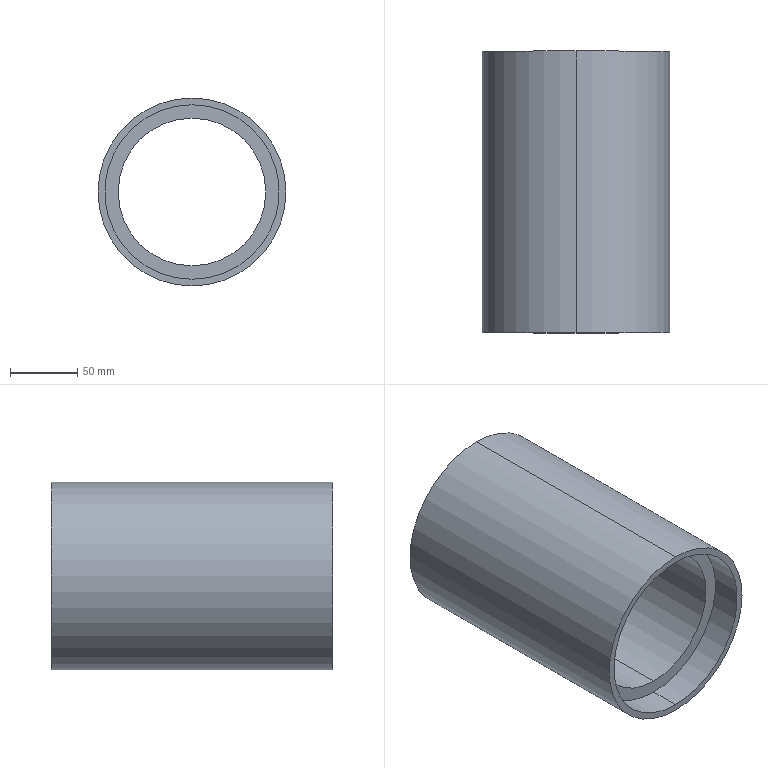Part | SolidWorks | features BaseBody 1 | 1 solid | 12 faces | box 140 x 210 x 140 mm | volume 1063586 mm3 | cylinder 8 | plane 4 | commonest cylinder face diameters 130 x4 110 x2 140 x2
STEP:
#1=CARTESIAN_POINT('',(0.,187.,-55.));
#2=VERTEX_POINT('',#1);
#3=CARTESIAN_POINT('',(0.,187.,55.));
#4=VERTEX_POINT('',#3);
#5=CARTESIAN_POINT('',(0.,187.,0.));
#6=DIRECTION('',(0.,1.,0.));
#7=DIRECTION('',(0.,0.,1.));
#8=AXIS2_PLACEMENT_3D('',#5,#6,#7);
#9=CIRCLE('',#8,55.);
#10=EDGE_CURVE('',#2,#4,#9,.T.);
#11=ORIENTED_EDGE('',*,*,#10,.T.);
#12=CARTESIAN_POINT('',(0.,23.,55.));
#13=VERTEX_POINT('',#12);
#14=CARTESIAN_POINT('',(0.,210.,55.));
#15=DIRECTION('',(0.,-1.,0.));
#16=VECTOR('',#15,1000.);
#17=LINE('',#14,#16);
#18=EDGE_CURVE('',#4,#13,#17,.T.);
#19=ORIENTED_EDGE('',*,*,#18,.T.);
#20=CARTESIAN_POINT('',(0.,23.,-55.));
#21=VERTEX_POINT('',#20);
#22=CARTESIAN_POINT('',(0.,23.,0.));
#23=DIRECTION('',(0.,-1.,0.));
#24=DIRECTION('',(0.,0.,-1.));
#25=AXIS2_PLACEMENT_3D('',#22,#23,#24);
#26=CIRCLE('',#25,55.);
#27=EDGE_CURVE('',#13,#21,#26,.T.);
#28=ORIENTED_EDGE('',*,*,#27,.T.);
#29=CARTESIAN_POINT('',(0.,210.,-55.));
#30=DIRECTION('',(0.,-1.,0.));
#31=VECTOR('',#30,1000.);
#32=LINE('',#29,#31);
#33=EDGE_CURVE('',#2,#21,#32,.T.);
#34=ORIENTED_EDGE('',*,*,#33,.F.);
#35=EDGE_LOOP('',(#11,#19,#28,#34));
#36=FACE_OUTER_BOUND('',#35,.T.);
#37=CARTESIAN_POINT('',(0.,210.,0.));
#38=DIRECTION('',(0.,-1.,0.));
#39=DIRECTION('',(0.,0.,-1.));
#40=AXIS2_PLACEMENT_3D('',#37,#38,#39);
#41=CYLINDRICAL_SURFACE('',#40,55.);
#42=ADVANCED_FACE('',(#36),#41,.F.);
#43=CARTESIAN_POINT('',(0.,23.,65.));
#44=VERTEX_POINT('',#43);
#45=CARTESIAN_POINT('',(0.,23.,-65.));
#46=VERTEX_POINT('',#45);
#47=CARTESIAN_POINT('',(0.,23.,0.));
#48=DIRECTION('',(0.,-1.,0.));
#49=DIRECTION('',(0.,0.,-1.));
#50=AXIS2_PLACEMENT_3D('',#47,#48,#49);
#51=CIRCLE('',#50,65.);
#52=EDGE_CURVE('',#44,#46,#51,.T.);
#53=ORIENTED_EDGE('',*,*,#52,.F.);
#54=CARTESIAN_POINT('',(0.,0.,65.));
#55=VERTEX_POINT('',#54);
#56=CARTESIAN_POINT('',(0.,23.,65.));
#57=DIRECTION('',(0.,-1.,0.));
#58=VECTOR('',#57,1000.);
#59=LINE('',#56,#58);
#60=EDGE_CURVE('',#44,#55,#59,.T.);
#61=ORIENTED_EDGE('',*,*,#60,.T.);
#62=CARTESIAN_POINT('',(0.,0.,-65.));
#63=VERTEX_POINT('',#62);
#64=CARTESIAN_POINT('',(0.,0.,0.));
#65=DIRECTION('',(0.,-1.,0.));
#66=DIRECTION('',(0.,0.,-1.));
#67=AXIS2_PLACEMENT_3D('',#64,#65,#66);
#68=CIRCLE('',#67,65.);
#69=EDGE_CURVE('',#55,#63,#68,.T.);
#70=ORIENTED_EDGE('',*,*,#69,.T.);
#71=CARTESIAN_POINT('',(0.,23.,-65.));
#72=DIRECTION('',(0.,-1.,0.));
#73=VECTOR('',#72,1000.);
#74=LINE('',#71,#73);
#75=EDGE_CURVE('',#46,#63,#74,.T.);
#76=ORIENTED_EDGE('',*,*,#75,.F.);
#77=EDGE_LOOP('',(#53,#61,#70,#76));
#78=FACE_OUTER_BOUND('',#77,.T.);
#79=CARTESIAN_POINT('',(0.,23.,0.));
#80=DIRECTION('',(0.,-1.,0.));
#81=DIRECTION('',(0.,0.,-1.));
#82=AXIS2_PLACEMENT_3D('',#79,#80,#81);
#83=CYLINDRICAL_SURFACE('',#82,65.);
#84=ADVANCED_FACE('',(#78),#83,.F.);
#85=CARTESIAN_POINT('',(0.,187.,-65.));
#86=VERTEX_POINT('',#85);
#87=CARTESIAN_POINT('',(0.,187.,65.));
#88=VERTEX_POINT('',#87);
#89=CARTESIAN_POINT('',(0.,187.,0.));
#90=DIRECTION('',(0.,1.,0.));
#91=DIRECTION('',(0.,0.,1.));
#92=AXIS2_PLACEMENT_3D('',#89,#90,#91);
#93=CIRCLE('',#92,65.);
#94=EDGE_CURVE('',#86,#88,#93,.T.);
#95=ORIENTED_EDGE('',*,*,#94,.F.);
#96=CARTESIAN_POINT('',(0.,210.,-65.));
#97=VERTEX_POINT('',#96);
#98=CARTESIAN_POINT('',(0.,187.,-65.));
#99=DIRECTION('',(0.,1.,0.));
#100=VECTOR('',#99,1000.);
#101=LINE('',#98,#100);
#102=EDGE_CURVE('',#86,#97,#101,.T.);
#103=ORIENTED_EDGE('',*,*,#102,.T.);
#104=CARTESIAN_POINT('',(0.,210.,65.));
#105=VERTEX_POINT('',#104);
#106=CARTESIAN_POINT('',(0.,210.,0.));
#107=DIRECTION('',(0.,1.,0.));
#108=DIRECTION('',(0.,0.,1.));
#109=AXIS2_PLACEMENT_3D('',#106,#107,#108);
#110=CIRCLE('',#109,65.);
#111=EDGE_CURVE('',#97,#105,#110,.T.);
#112=ORIENTED_EDGE('',*,*,#111,.T.);
#113=CARTESIAN_POINT('',(0.,187.,65.));
#114=DIRECTION('',(0.,1.,0.));
#115=VECTOR('',#114,1000.);
#116=LINE('',#113,#115);
#117=EDGE_CURVE('',#88,#105,#116,.T.);
#118=ORIENTED_EDGE('',*,*,#117,.F.);
#119=EDGE_LOOP('',(#95,#103,#112,#118));
#120=FACE_OUTER_BOUND('',#119,.T.);
#121=CARTESIAN_POINT('',(0.,187.,0.));
#122=DIRECTION('',(0.,1.,0.));
#123=DIRECTION('',(0.,0.,1.));
#124=AXIS2_PLACEMENT_3D('',#121,#122,#123);
#125=CYLINDRICAL_SURFACE('',#124,65.);
#126=ADVANCED_FACE('',(#120),#125,.F.);
#127=CARTESIAN_POINT('',(0.,210.,70.));
#128=VERTEX_POINT('',#127);
#129=CARTESIAN_POINT('',(0.,210.,-70.));
#130=VERTEX_POINT('',#129);
#131=CARTESIAN_POINT('',(0.,210.,0.));
#132=DIRECTION('',(0.,1.,0.));
#133=DIRECTION('',(0.,0.,1.));
#134=AXIS2_PLACEMENT_3D('',#131,#132,#133);
#135=CIRCLE('',#134,70.);
#136=EDGE_CURVE('',#128,#130,#135,.T.);
#137=ORIENTED_EDGE('',*,*,#136,.F.);
#138=CARTESIAN_POINT('',(0.,0.,70.));
#139=VERTEX_POINT('',#138);
#140=CARTESIAN_POINT('',(0.,210.,70.));
#141=DIRECTION('',(0.,-1.,0.));
#142=VECTOR('',#141,1000.);
#143=LINE('',#140,#142);
#144=EDGE_CURVE('',#128,#139,#143,.T.);
#145=ORIENTED_EDGE('',*,*,#144,.T.);
#146=CARTESIAN_POINT('',(0.,0.,-70.));
#147=VERTEX_POINT('',#146);
#148=CARTESIAN_POINT('',(0.,0.,0.));
#149=DIRECTION('',(0.,1.,0.));
#150=DIRECTION('',(0.,0.,1.));
#151=AXIS2_PLACEMENT_3D('',#148,#149,#150);
#152=CIRCLE('',#151,70.);
#153=EDGE_CURVE('',#139,#147,#152,.T.);
#154=ORIENTED_EDGE('',*,*,#153,.T.);
#155=CARTESIAN_POINT('',(0.,210.,-70.));
#156=DIRECTION('',(0.,-1.,0.));
#157=VECTOR('',#156,1000.);
#158=LINE('',#155,#157);
#159=EDGE_CURVE('',#130,#147,#158,.T.);
#160=ORIENTED_EDGE('',*,*,#159,.F.);
#161=EDGE_LOOP('',(#137,#145,#154,#160));
#162=FACE_OUTER_BOUND('',#161,.T.);
#163=CARTESIAN_POINT('',(0.,210.,0.));
#164=DIRECTION('',(0.,-1.,0.));
#165=DIRECTION('',(0.,0.,-1.));
#166=AXIS2_PLACEMENT_3D('',#163,#164,#165);
#167=CYLINDRICAL_SURFACE('',#166,70.);
#168=ADVANCED_FACE('',(#162),#167,.T.);
#169=ORIENTED_EDGE('',*,*,#144,.F.);
#170=CARTESIAN_POINT('',(0.,210.,0.));
#171=DIRECTION('',(0.,1.,0.));
#172=DIRECTION('',(0.,0.,1.));
#173=AXIS2_PLACEMENT_3D('',#170,#171,#172);
#174=CIRCLE('',#173,70.);
#175=EDGE_CURVE('',#130,#128,#174,.T.);
#176=ORIENTED_EDGE('',*,*,#175,.F.);
#177=ORIENTED_EDGE('',*,*,#159,.T.);
#178=CARTESIAN_POINT('',(0.,0.,0.));
#179=DIRECTION('',(0.,1.,0.));
#180=DIRECTION('',(0.,0.,1.));
#181=AXIS2_PLACEMENT_3D('',#178,#179,#180);
#182=CIRCLE('',#181,70.);
#183=EDGE_CURVE('',#147,#139,#182,.T.);
#184=ORIENTED_EDGE('',*,*,#183,.T.);
#185=EDGE_LOOP('',(#169,#176,#177,#184));
#186=FACE_OUTER_BOUND('',#185,.T.);
#187=CARTESIAN_POINT('',(0.,210.,0.));
#188=DIRECTION('',(0.,-1.,0.));
#189=DIRECTION('',(0.,0.,-1.));
#190=AXIS2_PLACEMENT_3D('',#187,#188,#189);
#191=CYLINDRICAL_SURFACE('',#190,70.);
#192=ADVANCED_FACE('',(#186),#191,.T.);
#193=CARTESIAN_POINT('',(0.,210.,0.));
#194=DIRECTION('',(0.,1.,0.));
#195=DIRECTION('',(0.,0.,1.));
#196=AXIS2_PLACEMENT_3D('',#193,#194,#195);
#197=CIRCLE('',#196,65.);
#198=EDGE_CURVE('',#105,#97,#197,.T.);
#199=ORIENTED_EDGE('',*,*,#198,.F.);
#200=ORIENTED_EDGE('',*,*,#111,.F.);
#201=EDGE_LOOP('',(#199,#200));
#202=FACE_BOUND('',#201,.T.);
#203=ORIENTED_EDGE('',*,*,#175,.T.);
#204=ORIENTED_EDGE('',*,*,#136,.T.);
#205=EDGE_LOOP('',(#203,#204));
#206=FACE_OUTER_BOUND('',#205,.T.);
#207=CARTESIAN_POINT('',(0.,210.,0.));
#208=DIRECTION('',(0.,1.,0.));
#209=DIRECTION('',(0.,0.,1.));
#210=AXIS2_PLACEMENT_3D('',#207,#208,#209);
#211=PLANE('',#210);
#212=ADVANCED_FACE('',(#202,#206),#211,.T.);
#213=CARTESIAN_POINT('',(0.,0.,0.));
#214=DIRECTION('',(0.,-1.,0.));
#215=DIRECTION('',(0.,0.,-1.));
#216=AXIS2_PLACEMENT_3D('',#213,#214,#215);
#217=CIRCLE('',#216,65.);
#218=EDGE_CURVE('',#63,#55,#217,.T.);
#219=ORIENTED_EDGE('',*,*,#218,.F.);
#220=ORIENTED_EDGE('',*,*,#69,.F.);
#221=EDGE_LOOP('',(#219,#220));
#222=FACE_BOUND('',#221,.T.);
#223=ORIENTED_EDGE('',*,*,#183,.F.);
#224=ORIENTED_EDGE('',*,*,#153,.F.);
#225=EDGE_LOOP('',(#223,#224));
#226=FACE_OUTER_BOUND('',#225,.T.);
#227=CARTESIAN_POINT('',(0.,0.,0.));
#228=DIRECTION('',(0.,1.,0.));
#229=DIRECTION('',(0.,0.,1.));
#230=AXIS2_PLACEMENT_3D('',#227,#228,#229);
#231=PLANE('',#230);
#232=ADVANCED_FACE('',(#222,#226),#231,.F.);
#233=ORIENTED_EDGE('',*,*,#102,.F.);
#234=CARTESIAN_POINT('',(0.,187.,0.));
#235=DIRECTION('',(0.,1.,0.));
#236=DIRECTION('',(0.,0.,1.));
#237=AXIS2_PLACEMENT_3D('',#234,#235,#236);
#238=CIRCLE('',#237,65.);
#239=EDGE_CURVE('',#88,#86,#238,.T.);
#240=ORIENTED_EDGE('',*,*,#239,.F.);
#241=ORIENTED_EDGE('',*,*,#117,.T.);
#242=ORIENTED_EDGE('',*,*,#198,.T.);
#243=EDGE_LOOP('',(#233,#240,#241,#242));
#244=FACE_OUTER_BOUND('',#243,.T.);
#245=CARTESIAN_POINT('',(0.,187.,0.));
#246=DIRECTION('',(0.,1.,0.));
#247=DIRECTION('',(0.,0.,1.));
#248=AXIS2_PLACEMENT_3D('',#245,#246,#247);
#249=CYLINDRICAL_SURFACE('',#248,65.);
#250=ADVANCED_FACE('',(#244),#249,.F.);
#251=ORIENTED_EDGE('',*,*,#10,.F.);
#252=CARTESIAN_POINT('',(0.,187.,0.));
#253=DIRECTION('',(0.,1.,0.));
#254=DIRECTION('',(0.,0.,1.));
#255=AXIS2_PLACEMENT_3D('',#252,#253,#254);
#256=CIRCLE('',#255,55.);
#257=EDGE_CURVE('',#4,#2,#256,.T.);
#258=ORIENTED_EDGE('',*,*,#257,.F.);
#259=EDGE_LOOP('',(#251,#258));
#260=FACE_BOUND('',#259,.T.);
#261=ORIENTED_EDGE('',*,*,#239,.T.);
#262=ORIENTED_EDGE('',*,*,#94,.T.);
#263=EDGE_LOOP('',(#261,#262));
#264=FACE_OUTER_BOUND('',#263,.T.);
#265=CARTESIAN_POINT('',(0.,187.,0.));
#266=DIRECTION('',(0.,1.,0.));
#267=DIRECTION('',(0.,0.,1.));
#268=AXIS2_PLACEMENT_3D('',#265,#266,#267);
#269=PLANE('',#268);
#270=ADVANCED_FACE('',(#260,#264),#269,.T.);
#271=ORIENTED_EDGE('',*,*,#60,.F.);
#272=CARTESIAN_POINT('',(0.,23.,0.));
#273=DIRECTION('',(0.,-1.,0.));
#274=DIRECTION('',(0.,0.,-1.));
#275=AXIS2_PLACEMENT_3D('',#272,#273,#274);
#276=CIRCLE('',#275,65.);
#277=EDGE_CURVE('',#46,#44,#276,.T.);
#278=ORIENTED_EDGE('',*,*,#277,.F.);
#279=ORIENTED_EDGE('',*,*,#75,.T.);
#280=ORIENTED_EDGE('',*,*,#218,.T.);
#281=EDGE_LOOP('',(#271,#278,#279,#280));
#282=FACE_OUTER_BOUND('',#281,.T.);
#283=CARTESIAN_POINT('',(0.,23.,0.));
#284=DIRECTION('',(0.,-1.,0.));
#285=DIRECTION('',(0.,0.,-1.));
#286=AXIS2_PLACEMENT_3D('',#283,#284,#285);
#287=CYLINDRICAL_SURFACE('',#286,65.);
#288=ADVANCED_FACE('',(#282),#287,.F.);
#289=CARTESIAN_POINT('',(0.,23.,0.));
#290=DIRECTION('',(0.,-1.,0.));
#291=DIRECTION('',(0.,0.,-1.));
#292=AXIS2_PLACEMENT_3D('',#289,#290,#291);
#293=CIRCLE('',#292,55.);
#294=EDGE_CURVE('',#21,#13,#293,.T.);
#295=ORIENTED_EDGE('',*,*,#294,.F.);
#296=ORIENTED_EDGE('',*,*,#27,.F.);
#297=EDGE_LOOP('',(#295,#296));
#298=FACE_BOUND('',#297,.T.);
#299=ORIENTED_EDGE('',*,*,#277,.T.);
#300=ORIENTED_EDGE('',*,*,#52,.T.);
#301=EDGE_LOOP('',(#299,#300));
#302=FACE_OUTER_BOUND('',#301,.T.);
#303=CARTESIAN_POINT('',(0.,23.,0.));
#304=DIRECTION('',(0.,-1.,0.));
#305=DIRECTION('',(0.,0.,-1.));
#306=AXIS2_PLACEMENT_3D('',#303,#304,#305);
#307=PLANE('',#306);
#308=ADVANCED_FACE('',(#298,#302),#307,.T.);
#309=ORIENTED_EDGE('',*,*,#18,.F.);
#310=ORIENTED_EDGE('',*,*,#257,.T.);
#311=ORIENTED_EDGE('',*,*,#33,.T.);
#312=ORIENTED_EDGE('',*,*,#294,.T.);
#313=EDGE_LOOP('',(#309,#310,#311,#312));
#314=FACE_OUTER_BOUND('',#313,.T.);
#315=CARTESIAN_POINT('',(0.,210.,0.));
#316=DIRECTION('',(0.,-1.,0.));
#317=DIRECTION('',(0.,0.,-1.));
#318=AXIS2_PLACEMENT_3D('',#315,#316,#317);
#319=CYLINDRICAL_SURFACE('',#318,55.);
#320=ADVANCED_FACE('',(#314),#319,.F.);
#321=CLOSED_SHELL('',(#42,#84,#126,#168,#192,#212,#232,#250,#270,#288,#308,#320));
#322=MANIFOLD_SOLID_BREP('',#321);
#323=CARTESIAN_POINT('',(0.,0.,0.));
#324=DIRECTION('',(0.,0.,1.));
#325=DIRECTION('',(1.,0.,0.));
#326=AXIS2_PLACEMENT_3D('',#323,#324,#325);
#327=(LENGTH_UNIT()NAMED_UNIT(*)SI_UNIT(.MILLI.,.METRE.));
#328=UNCERTAINTY_MEASURE_WITH_UNIT(LENGTH_MEASURE(0.00001),#327,'','');
#329=(NAMED_UNIT(*)PLANE_ANGLE_UNIT()SI_UNIT($,.RADIAN.));
#330=(NAMED_UNIT(*)SI_UNIT($,.STERADIAN.)SOLID_ANGLE_UNIT());
#331=(GEOMETRIC_REPRESENTATION_CONTEXT(3)GLOBAL_UNCERTAINTY_ASSIGNED_CONTEXT((#328))GLOBAL_UNIT_ASSIGNED_CONTEXT((#327,#329,#330))REPRESENTATION_CONTEXT('',''));
#332=ADVANCED_BREP_SHAPE_REPRESENTATION('',(#322,#326),#331);